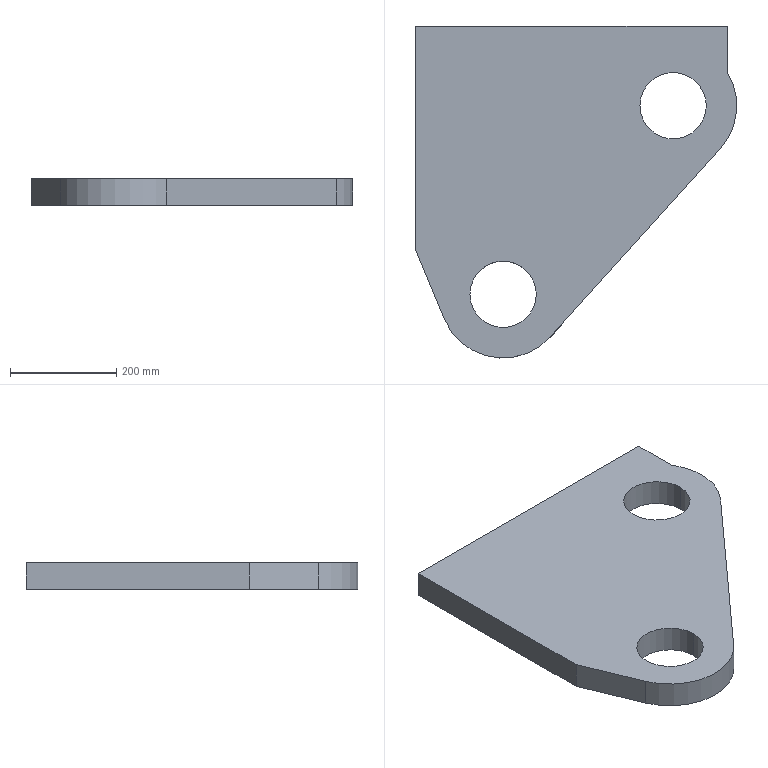Part | SolidWorks | features SplitBody 1 | 1 solid | 13 faces | box 605 x 625 x 50 mm | volume 12914226 mm3 | plane 7 | cylinder 6 | commonest cylinder face diameters 125 x4 240 x2
STEP:
#1=CARTESIAN_POINT('',(3178.5,413.44,-755.));
#2=VERTEX_POINT('',#1);
#3=CARTESIAN_POINT('',(3053.5,413.44,-755.));
#4=VERTEX_POINT('',#3);
#5=CARTESIAN_POINT('',(3116.,413.44,-755.));
#6=DIRECTION('',(0.,0.,-1.));
#7=DIRECTION('',(-1.,0.,0.));
#8=AXIS2_PLACEMENT_3D('',#5,#6,#7);
#9=CIRCLE('',#8,62.5);
#10=EDGE_CURVE('',#2,#4,#9,.T.);
#11=ORIENTED_EDGE('',*,*,#10,.F.);
#12=CARTESIAN_POINT('',(3178.5,413.44,-805.));
#13=VERTEX_POINT('',#12);
#14=CARTESIAN_POINT('',(3178.5,413.44,-755.));
#15=DIRECTION('',(0.,0.,-1.));
#16=VECTOR('',#15,1000.);
#17=LINE('',#14,#16);
#18=EDGE_CURVE('',#2,#13,#17,.T.);
#19=ORIENTED_EDGE('',*,*,#18,.T.);
#20=CARTESIAN_POINT('',(3053.5,413.44,-805.));
#21=VERTEX_POINT('',#20);
#22=CARTESIAN_POINT('',(3116.,413.44,-805.));
#23=DIRECTION('',(0.,0.,1.));
#24=DIRECTION('',(-1.,0.,0.));
#25=AXIS2_PLACEMENT_3D('',#22,#23,#24);
#26=CIRCLE('',#25,62.5);
#27=EDGE_CURVE('',#21,#13,#26,.T.);
#28=ORIENTED_EDGE('',*,*,#27,.F.);
#29=CARTESIAN_POINT('',(3053.5,413.44,-755.));
#30=DIRECTION('',(0.,0.,-1.));
#31=VECTOR('',#30,1000.);
#32=LINE('',#29,#31);
#33=EDGE_CURVE('',#4,#21,#32,.T.);
#34=ORIENTED_EDGE('',*,*,#33,.F.);
#35=EDGE_LOOP('',(#11,#19,#28,#34));
#36=FACE_OUTER_BOUND('',#35,.T.);
#37=CARTESIAN_POINT('',(3116.,413.44,-755.));
#38=DIRECTION('',(0.,0.,-1.));
#39=DIRECTION('',(-1.,0.,0.));
#40=AXIS2_PLACEMENT_3D('',#37,#38,#39);
#41=CYLINDRICAL_SURFACE('',#40,62.5);
#42=ADVANCED_FACE('',(#36),#41,.F.);
#43=CARTESIAN_POINT('',(3498.5,768.44,-755.));
#44=VERTEX_POINT('',#43);
#45=CARTESIAN_POINT('',(3373.5,768.44,-755.));
#46=VERTEX_POINT('',#45);
#47=CARTESIAN_POINT('',(3436.,768.44,-755.));
#48=DIRECTION('',(0.,0.,-1.));
#49=DIRECTION('',(-1.,0.,0.));
#50=AXIS2_PLACEMENT_3D('',#47,#48,#49);
#51=CIRCLE('',#50,62.5);
#52=EDGE_CURVE('',#44,#46,#51,.T.);
#53=ORIENTED_EDGE('',*,*,#52,.F.);
#54=CARTESIAN_POINT('',(3498.5,768.44,-805.));
#55=VERTEX_POINT('',#54);
#56=CARTESIAN_POINT('',(3498.5,768.44,-755.));
#57=DIRECTION('',(0.,0.,-1.));
#58=VECTOR('',#57,1000.);
#59=LINE('',#56,#58);
#60=EDGE_CURVE('',#44,#55,#59,.T.);
#61=ORIENTED_EDGE('',*,*,#60,.T.);
#62=CARTESIAN_POINT('',(3373.5,768.44,-805.));
#63=VERTEX_POINT('',#62);
#64=CARTESIAN_POINT('',(3436.,768.44,-805.));
#65=DIRECTION('',(0.,0.,1.));
#66=DIRECTION('',(-1.,0.,0.));
#67=AXIS2_PLACEMENT_3D('',#64,#65,#66);
#68=CIRCLE('',#67,62.5);
#69=EDGE_CURVE('',#63,#55,#68,.T.);
#70=ORIENTED_EDGE('',*,*,#69,.F.);
#71=CARTESIAN_POINT('',(3373.5,768.44,-755.));
#72=DIRECTION('',(0.,0.,-1.));
#73=VECTOR('',#72,1000.);
#74=LINE('',#71,#73);
#75=EDGE_CURVE('',#46,#63,#74,.T.);
#76=ORIENTED_EDGE('',*,*,#75,.F.);
#77=EDGE_LOOP('',(#53,#61,#70,#76));
#78=FACE_OUTER_BOUND('',#77,.T.);
#79=CARTESIAN_POINT('',(3436.,768.44,-755.));
#80=DIRECTION('',(0.,0.,-1.));
#81=DIRECTION('',(-1.,0.,0.));
#82=AXIS2_PLACEMENT_3D('',#79,#80,#81);
#83=CYLINDRICAL_SURFACE('',#82,62.5);
#84=ADVANCED_FACE('',(#78),#83,.F.);
#85=CARTESIAN_POINT('',(3116.,413.44,-755.));
#86=DIRECTION('',(0.,0.,-1.));
#87=DIRECTION('',(-1.,0.,0.));
#88=AXIS2_PLACEMENT_3D('',#85,#86,#87);
#89=CIRCLE('',#88,62.5);
#90=EDGE_CURVE('',#4,#2,#89,.T.);
#91=ORIENTED_EDGE('',*,*,#90,.T.);
#92=ORIENTED_EDGE('',*,*,#10,.T.);
#93=EDGE_LOOP('',(#91,#92));
#94=FACE_BOUND('',#93,.T.);
#95=CARTESIAN_POINT('',(2951.,918.44,-755.));
#96=VERTEX_POINT('',#95);
#97=CARTESIAN_POINT('',(2951.,498.44,-755.));
#98=VERTEX_POINT('',#97);
#99=CARTESIAN_POINT('',(2951.,413.44,-755.));
#100=DIRECTION('',(0.,-1.,0.));
#101=VECTOR('',#100,1000.);
#102=LINE('',#99,#101);
#103=EDGE_CURVE('',#96,#98,#102,.T.);
#104=ORIENTED_EDGE('',*,*,#103,.T.);
#105=CARTESIAN_POINT('',(3005.106,367.587,-755.));
#106=VERTEX_POINT('',#105);
#107=CARTESIAN_POINT('',(2951.,498.44,-755.));
#108=DIRECTION('',(0.3821,-0.9241,0.));
#109=VECTOR('',#108,1000.);
#110=LINE('',#107,#109);
#111=EDGE_CURVE('',#98,#106,#110,.T.);
#112=ORIENTED_EDGE('',*,*,#111,.T.);
#113=CARTESIAN_POINT('',(3205.133,333.095,-755.));
#114=VERTEX_POINT('',#113);
#115=CARTESIAN_POINT('',(3116.,413.44,-755.));
#116=DIRECTION('',(0.,0.,1.));
#117=DIRECTION('',(-1.,0.,0.));
#118=AXIS2_PLACEMENT_3D('',#115,#116,#117);
#119=CIRCLE('',#118,120.);
#120=EDGE_CURVE('',#106,#114,#119,.T.);
#121=ORIENTED_EDGE('',*,*,#120,.T.);
#122=CARTESIAN_POINT('',(3525.133,688.095,-755.));
#123=VERTEX_POINT('',#122);
#124=CARTESIAN_POINT('',(3205.133,333.095,-755.));
#125=DIRECTION('',(0.6695,0.7428,0.));
#126=VECTOR('',#125,1000.);
#127=LINE('',#124,#126);
#128=EDGE_CURVE('',#114,#123,#127,.T.);
#129=ORIENTED_EDGE('',*,*,#128,.T.);
#130=CARTESIAN_POINT('',(3538.,831.654,-755.));
#131=VERTEX_POINT('',#130);
#132=CARTESIAN_POINT('',(3436.,768.44,-755.));
#133=DIRECTION('',(0.,0.,1.));
#134=DIRECTION('',(-1.,0.,0.));
#135=AXIS2_PLACEMENT_3D('',#132,#133,#134);
#136=CIRCLE('',#135,120.);
#137=EDGE_CURVE('',#123,#131,#136,.T.);
#138=ORIENTED_EDGE('',*,*,#137,.T.);
#139=CARTESIAN_POINT('',(3538.,918.44,-755.));
#140=VERTEX_POINT('',#139);
#141=CARTESIAN_POINT('',(3538.,413.44,-755.));
#142=DIRECTION('',(0.,1.,0.));
#143=VECTOR('',#142,1000.);
#144=LINE('',#141,#143);
#145=EDGE_CURVE('',#131,#140,#144,.T.);
#146=ORIENTED_EDGE('',*,*,#145,.T.);
#147=CARTESIAN_POINT('',(3116.,918.44,-755.));
#148=DIRECTION('',(-1.,0.,0.));
#149=VECTOR('',#148,1000.);
#150=LINE('',#147,#149);
#151=EDGE_CURVE('',#140,#96,#150,.T.);
#152=ORIENTED_EDGE('',*,*,#151,.T.);
#153=EDGE_LOOP('',(#104,#112,#121,#129,#138,#146,#152));
#154=FACE_OUTER_BOUND('',#153,.T.);
#155=CARTESIAN_POINT('',(3436.,768.44,-755.));
#156=DIRECTION('',(0.,0.,-1.));
#157=DIRECTION('',(-1.,0.,0.));
#158=AXIS2_PLACEMENT_3D('',#155,#156,#157);
#159=CIRCLE('',#158,62.5);
#160=EDGE_CURVE('',#46,#44,#159,.T.);
#161=ORIENTED_EDGE('',*,*,#160,.T.);
#162=ORIENTED_EDGE('',*,*,#52,.T.);
#163=EDGE_LOOP('',(#161,#162));
#164=FACE_BOUND('',#163,.T.);
#165=CARTESIAN_POINT('',(3116.,413.44,-755.));
#166=DIRECTION('',(0.,0.,1.));
#167=DIRECTION('',(1.,0.,0.));
#168=AXIS2_PLACEMENT_3D('',#165,#166,#167);
#169=PLANE('',#168);
#170=ADVANCED_FACE('',(#94,#154,#164),#169,.T.);
#171=ORIENTED_EDGE('',*,*,#18,.F.);
#172=ORIENTED_EDGE('',*,*,#90,.F.);
#173=ORIENTED_EDGE('',*,*,#33,.T.);
#174=CARTESIAN_POINT('',(3116.,413.44,-805.));
#175=DIRECTION('',(0.,0.,1.));
#176=DIRECTION('',(-1.,0.,0.));
#177=AXIS2_PLACEMENT_3D('',#174,#175,#176);
#178=CIRCLE('',#177,62.5);
#179=EDGE_CURVE('',#13,#21,#178,.T.);
#180=ORIENTED_EDGE('',*,*,#179,.F.);
#181=EDGE_LOOP('',(#171,#172,#173,#180));
#182=FACE_OUTER_BOUND('',#181,.T.);
#183=CARTESIAN_POINT('',(3116.,413.44,-755.));
#184=DIRECTION('',(0.,0.,-1.));
#185=DIRECTION('',(-1.,0.,0.));
#186=AXIS2_PLACEMENT_3D('',#183,#184,#185);
#187=CYLINDRICAL_SURFACE('',#186,62.5);
#188=ADVANCED_FACE('',(#182),#187,.F.);
#189=CARTESIAN_POINT('',(3005.106,367.587,-805.));
#190=VERTEX_POINT('',#189);
#191=CARTESIAN_POINT('',(3005.106,367.587,-755.));
#192=DIRECTION('',(0.,0.,-1.));
#193=VECTOR('',#192,1000.);
#194=LINE('',#191,#193);
#195=EDGE_CURVE('',#106,#190,#194,.T.);
#196=ORIENTED_EDGE('',*,*,#195,.F.);
#197=ORIENTED_EDGE('',*,*,#111,.F.);
#198=CARTESIAN_POINT('',(2951.,498.44,-805.));
#199=VERTEX_POINT('',#198);
#200=CARTESIAN_POINT('',(2951.,498.44,-755.));
#201=DIRECTION('',(0.,0.,1.));
#202=VECTOR('',#201,1000.);
#203=LINE('',#200,#202);
#204=EDGE_CURVE('',#199,#98,#203,.T.);
#205=ORIENTED_EDGE('',*,*,#204,.F.);
#206=CARTESIAN_POINT('',(2951.,498.44,-805.));
#207=DIRECTION('',(-0.3821,0.9241,0.));
#208=VECTOR('',#207,1000.);
#209=LINE('',#206,#208);
#210=EDGE_CURVE('',#190,#199,#209,.T.);
#211=ORIENTED_EDGE('',*,*,#210,.F.);
#212=EDGE_LOOP('',(#196,#197,#205,#211));
#213=FACE_OUTER_BOUND('',#212,.T.);
#214=CARTESIAN_POINT('',(2951.,498.44,-755.));
#215=DIRECTION('',(0.9241,0.3821,0.));
#216=DIRECTION('',(-0.3821,0.9241,0.));
#217=AXIS2_PLACEMENT_3D('',#214,#215,#216);
#218=PLANE('',#217);
#219=ADVANCED_FACE('',(#213),#218,.F.);
#220=ORIENTED_EDGE('',*,*,#204,.T.);
#221=ORIENTED_EDGE('',*,*,#103,.F.);
#222=CARTESIAN_POINT('',(2951.,918.44,-805.));
#223=VERTEX_POINT('',#222);
#224=CARTESIAN_POINT('',(2951.,918.44,-755.));
#225=DIRECTION('',(0.,0.,1.));
#226=VECTOR('',#225,1000.);
#227=LINE('',#224,#226);
#228=EDGE_CURVE('',#223,#96,#227,.T.);
#229=ORIENTED_EDGE('',*,*,#228,.F.);
#230=CARTESIAN_POINT('',(2951.,498.44,-805.));
#231=DIRECTION('',(0.,1.,0.));
#232=VECTOR('',#231,1000.);
#233=LINE('',#230,#232);
#234=EDGE_CURVE('',#199,#223,#233,.T.);
#235=ORIENTED_EDGE('',*,*,#234,.F.);
#236=EDGE_LOOP('',(#220,#221,#229,#235));
#237=FACE_OUTER_BOUND('',#236,.T.);
#238=CARTESIAN_POINT('',(2951.,498.44,-755.));
#239=DIRECTION('',(1.,0.,0.));
#240=DIRECTION('',(0.,0.,-1.));
#241=AXIS2_PLACEMENT_3D('',#238,#239,#240);
#242=PLANE('',#241);
#243=ADVANCED_FACE('',(#237),#242,.F.);
#244=ORIENTED_EDGE('',*,*,#228,.T.);
#245=ORIENTED_EDGE('',*,*,#151,.F.);
#246=CARTESIAN_POINT('',(3538.,918.44,-805.));
#247=VERTEX_POINT('',#246);
#248=CARTESIAN_POINT('',(3538.,918.44,-755.));
#249=DIRECTION('',(0.,0.,1.));
#250=VECTOR('',#249,1000.);
#251=LINE('',#248,#250);
#252=EDGE_CURVE('',#247,#140,#251,.T.);
#253=ORIENTED_EDGE('',*,*,#252,.F.);
#254=CARTESIAN_POINT('',(2951.,918.44,-805.));
#255=DIRECTION('',(1.,0.,0.));
#256=VECTOR('',#255,1000.);
#257=LINE('',#254,#256);
#258=EDGE_CURVE('',#223,#247,#257,.T.);
#259=ORIENTED_EDGE('',*,*,#258,.F.);
#260=EDGE_LOOP('',(#244,#245,#253,#259));
#261=FACE_OUTER_BOUND('',#260,.T.);
#262=CARTESIAN_POINT('',(2951.,918.44,-755.));
#263=DIRECTION('',(0.,-1.,0.));
#264=DIRECTION('',(1.,0.,0.));
#265=AXIS2_PLACEMENT_3D('',#262,#263,#264);
#266=PLANE('',#265);
#267=ADVANCED_FACE('',(#261),#266,.F.);
#268=ORIENTED_EDGE('',*,*,#252,.T.);
#269=ORIENTED_EDGE('',*,*,#145,.F.);
#270=CARTESIAN_POINT('',(3538.,831.654,-805.));
#271=VERTEX_POINT('',#270);
#272=CARTESIAN_POINT('',(3538.,831.654,-755.));
#273=DIRECTION('',(0.,0.,1.));
#274=VECTOR('',#273,1000.);
#275=LINE('',#272,#274);
#276=EDGE_CURVE('',#271,#131,#275,.T.);
#277=ORIENTED_EDGE('',*,*,#276,.F.);
#278=CARTESIAN_POINT('',(3538.,918.44,-805.));
#279=DIRECTION('',(0.,-1.,0.));
#280=VECTOR('',#279,1000.);
#281=LINE('',#278,#280);
#282=EDGE_CURVE('',#247,#271,#281,.T.);
#283=ORIENTED_EDGE('',*,*,#282,.F.);
#284=EDGE_LOOP('',(#268,#269,#277,#283));
#285=FACE_OUTER_BOUND('',#284,.T.);
#286=CARTESIAN_POINT('',(3538.,918.44,-755.));
#287=DIRECTION('',(-1.,0.,0.));
#288=DIRECTION('',(0.,-1.,0.));
#289=AXIS2_PLACEMENT_3D('',#286,#287,#288);
#290=PLANE('',#289);
#291=ADVANCED_FACE('',(#285),#290,.F.);
#292=ORIENTED_EDGE('',*,*,#137,.F.);
#293=CARTESIAN_POINT('',(3525.133,688.095,-805.));
#294=VERTEX_POINT('',#293);
#295=CARTESIAN_POINT('',(3525.133,688.095,-755.));
#296=DIRECTION('',(0.,0.,-1.));
#297=VECTOR('',#296,1000.);
#298=LINE('',#295,#297);
#299=EDGE_CURVE('',#123,#294,#298,.T.);
#300=ORIENTED_EDGE('',*,*,#299,.T.);
#301=CARTESIAN_POINT('',(3436.,768.44,-805.));
#302=DIRECTION('',(0.,0.,1.));
#303=DIRECTION('',(-1.,0.,0.));
#304=AXIS2_PLACEMENT_3D('',#301,#302,#303);
#305=CIRCLE('',#304,120.);
#306=EDGE_CURVE('',#294,#271,#305,.T.);
#307=ORIENTED_EDGE('',*,*,#306,.T.);
#308=ORIENTED_EDGE('',*,*,#276,.T.);
#309=EDGE_LOOP('',(#292,#300,#307,#308));
#310=FACE_OUTER_BOUND('',#309,.T.);
#311=CARTESIAN_POINT('',(3436.,768.44,-755.));
#312=DIRECTION('',(0.,0.,-1.));
#313=DIRECTION('',(-1.,0.,0.));
#314=AXIS2_PLACEMENT_3D('',#311,#312,#313);
#315=CYLINDRICAL_SURFACE('',#314,120.);
#316=ADVANCED_FACE('',(#310),#315,.T.);
#317=ORIENTED_EDGE('',*,*,#299,.F.);
#318=ORIENTED_EDGE('',*,*,#128,.F.);
#319=CARTESIAN_POINT('',(3205.133,333.095,-805.));
#320=VERTEX_POINT('',#319);
#321=CARTESIAN_POINT('',(3205.133,333.095,-755.));
#322=DIRECTION('',(0.,0.,1.));
#323=VECTOR('',#322,1000.);
#324=LINE('',#321,#323);
#325=EDGE_CURVE('',#320,#114,#324,.T.);
#326=ORIENTED_EDGE('',*,*,#325,.F.);
#327=CARTESIAN_POINT('',(3205.133,333.095,-805.));
#328=DIRECTION('',(-0.6695,-0.7428,0.));
#329=VECTOR('',#328,1000.);
#330=LINE('',#327,#329);
#331=EDGE_CURVE('',#294,#320,#330,.T.);
#332=ORIENTED_EDGE('',*,*,#331,.F.);
#333=EDGE_LOOP('',(#317,#318,#326,#332));
#334=FACE_OUTER_BOUND('',#333,.T.);
#335=CARTESIAN_POINT('',(3205.133,333.095,-755.));
#336=DIRECTION('',(-0.7428,0.6695,0.));
#337=DIRECTION('',(-0.6695,-0.7428,0.));
#338=AXIS2_PLACEMENT_3D('',#335,#336,#337);
#339=PLANE('',#338);
#340=ADVANCED_FACE('',(#334),#339,.F.);
#341=ORIENTED_EDGE('',*,*,#120,.F.);
#342=ORIENTED_EDGE('',*,*,#195,.T.);
#343=CARTESIAN_POINT('',(3116.,413.44,-805.));
#344=DIRECTION('',(0.,0.,1.));
#345=DIRECTION('',(-1.,0.,0.));
#346=AXIS2_PLACEMENT_3D('',#343,#344,#345);
#347=CIRCLE('',#346,120.);
#348=EDGE_CURVE('',#190,#320,#347,.T.);
#349=ORIENTED_EDGE('',*,*,#348,.T.);
#350=ORIENTED_EDGE('',*,*,#325,.T.);
#351=EDGE_LOOP('',(#341,#342,#349,#350));
#352=FACE_OUTER_BOUND('',#351,.T.);
#353=CARTESIAN_POINT('',(3116.,413.44,-755.));
#354=DIRECTION('',(0.,0.,-1.));
#355=DIRECTION('',(-1.,0.,0.));
#356=AXIS2_PLACEMENT_3D('',#353,#354,#355);
#357=CYLINDRICAL_SURFACE('',#356,120.);
#358=ADVANCED_FACE('',(#352),#357,.T.);
#359=ORIENTED_EDGE('',*,*,#60,.F.);
#360=ORIENTED_EDGE('',*,*,#160,.F.);
#361=ORIENTED_EDGE('',*,*,#75,.T.);
#362=CARTESIAN_POINT('',(3436.,768.44,-805.));
#363=DIRECTION('',(0.,0.,1.));
#364=DIRECTION('',(-1.,0.,0.));
#365=AXIS2_PLACEMENT_3D('',#362,#363,#364);
#366=CIRCLE('',#365,62.5);
#367=EDGE_CURVE('',#55,#63,#366,.T.);
#368=ORIENTED_EDGE('',*,*,#367,.F.);
#369=EDGE_LOOP('',(#359,#360,#361,#368));
#370=FACE_OUTER_BOUND('',#369,.T.);
#371=CARTESIAN_POINT('',(3436.,768.44,-755.));
#372=DIRECTION('',(0.,0.,-1.));
#373=DIRECTION('',(-1.,0.,0.));
#374=AXIS2_PLACEMENT_3D('',#371,#372,#373);
#375=CYLINDRICAL_SURFACE('',#374,62.5);
#376=ADVANCED_FACE('',(#370),#375,.F.);
#377=ORIENTED_EDGE('',*,*,#27,.T.);
#378=ORIENTED_EDGE('',*,*,#179,.T.);
#379=EDGE_LOOP('',(#377,#378));
#380=FACE_BOUND('',#379,.T.);
#381=ORIENTED_EDGE('',*,*,#210,.T.);
#382=ORIENTED_EDGE('',*,*,#234,.T.);
#383=ORIENTED_EDGE('',*,*,#258,.T.);
#384=ORIENTED_EDGE('',*,*,#282,.T.);
#385=ORIENTED_EDGE('',*,*,#306,.F.);
#386=ORIENTED_EDGE('',*,*,#331,.T.);
#387=ORIENTED_EDGE('',*,*,#348,.F.);
#388=EDGE_LOOP('',(#381,#382,#383,#384,#385,#386,#387));
#389=FACE_OUTER_BOUND('',#388,.T.);
#390=ORIENTED_EDGE('',*,*,#69,.T.);
#391=ORIENTED_EDGE('',*,*,#367,.T.);
#392=EDGE_LOOP('',(#390,#391));
#393=FACE_BOUND('',#392,.T.);
#394=CARTESIAN_POINT('',(3116.,413.44,-805.));
#395=DIRECTION('',(0.,0.,1.));
#396=DIRECTION('',(1.,0.,0.));
#397=AXIS2_PLACEMENT_3D('',#394,#395,#396);
#398=PLANE('',#397);
#399=ADVANCED_FACE('',(#380,#389,#393),#398,.F.);
#400=CLOSED_SHELL('',(#42,#84,#170,#188,#219,#243,#267,#291,#316,#340,#358,#376,#399));
#401=MANIFOLD_SOLID_BREP('',#400);
#402=CARTESIAN_POINT('',(0.,0.,0.));
#403=DIRECTION('',(0.,0.,1.));
#404=DIRECTION('',(1.,0.,0.));
#405=AXIS2_PLACEMENT_3D('',#402,#403,#404);
#406=(LENGTH_UNIT()NAMED_UNIT(*)SI_UNIT(.MILLI.,.METRE.));
#407=UNCERTAINTY_MEASURE_WITH_UNIT(LENGTH_MEASURE(0.00001),#406,'','');
#408=(NAMED_UNIT(*)PLANE_ANGLE_UNIT()SI_UNIT($,.RADIAN.));
#409=(NAMED_UNIT(*)SI_UNIT($,.STERADIAN.)SOLID_ANGLE_UNIT());
#410=(GEOMETRIC_REPRESENTATION_CONTEXT(3)GLOBAL_UNCERTAINTY_ASSIGNED_CONTEXT((#407))GLOBAL_UNIT_ASSIGNED_CONTEXT((#406,#408,#409))REPRESENTATION_CONTEXT('',''));
#411=ADVANCED_BREP_SHAPE_REPRESENTATION('',(#401,#405),#410);